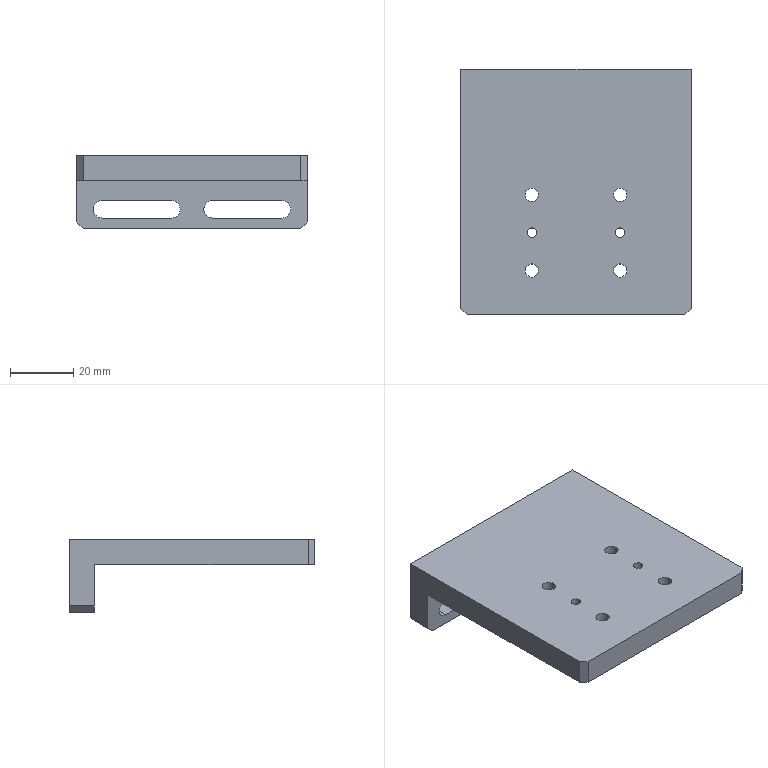Part | STEP file | 11-FG-SZ02611 | 1 solid | 34 faces | box 73 x 77.8 x 23 mm | volume 51259 mm3 | cylinder 18 | plane 16 | commonest cylinder face diameters 4.2 x8 5.5 x6 3 x4
STEP:
#1=CARTESIAN_POINT('',(-3.75,38.9,-9.));
#2=VERTEX_POINT('',#1);
#3=CARTESIAN_POINT('',(-6.5,38.9,-6.25));
#4=VERTEX_POINT('',#3);
#5=CARTESIAN_POINT('',(-6.5,38.9,-9.));
#6=DIRECTION('',(0.,-1.,0.));
#7=DIRECTION('',(0.,0.,-1.));
#8=AXIS2_PLACEMENT_3D('',#5,#6,#7);
#9=CIRCLE('',#8,2.75);
#10=EDGE_CURVE('',#2,#4,#9,.T.);
#11=ORIENTED_EDGE('',*,*,#10,.F.);
#12=CARTESIAN_POINT('',(-3.75,30.9,-9.));
#13=VERTEX_POINT('',#12);
#14=CARTESIAN_POINT('',(-3.75,53.9,-9.));
#15=DIRECTION('',(0.,-1.,0.));
#16=VECTOR('',#15,1000.);
#17=LINE('',#14,#16);
#18=EDGE_CURVE('',#2,#13,#17,.T.);
#19=ORIENTED_EDGE('',*,*,#18,.T.);
#20=CARTESIAN_POINT('',(-6.5,30.9,-6.25));
#21=VERTEX_POINT('',#20);
#22=CARTESIAN_POINT('',(-6.5,30.9,-9.));
#23=DIRECTION('',(0.,-1.,0.));
#24=DIRECTION('',(1.,0.,0.));
#25=AXIS2_PLACEMENT_3D('',#22,#23,#24);
#26=CIRCLE('',#25,2.75);
#27=EDGE_CURVE('',#13,#21,#26,.T.);
#28=ORIENTED_EDGE('',*,*,#27,.T.);
#29=CARTESIAN_POINT('',(-6.5,53.9,-6.25));
#30=DIRECTION('',(0.,-1.,0.));
#31=VECTOR('',#30,1000.);
#32=LINE('',#29,#31);
#33=EDGE_CURVE('',#4,#21,#32,.T.);
#34=ORIENTED_EDGE('',*,*,#33,.F.);
#35=EDGE_LOOP('',(#11,#19,#28,#34));
#36=FACE_OUTER_BOUND('',#35,.T.);
#37=CARTESIAN_POINT('',(-6.5,53.9,-9.));
#38=DIRECTION('',(0.,-1.,0.));
#39=DIRECTION('',(1.,0.,0.));
#40=AXIS2_PLACEMENT_3D('',#37,#38,#39);
#41=CYLINDRICAL_SURFACE('',#40,2.75);
#42=ADVANCED_FACE('',(#36),#41,.F.);
#43=CARTESIAN_POINT('',(-15.5,-12.9,8.));
#44=VERTEX_POINT('',#43);
#45=CARTESIAN_POINT('',(-12.5,-12.9,8.));
#46=VERTEX_POINT('',#45);
#47=CARTESIAN_POINT('',(-14.,-12.9,8.));
#48=DIRECTION('',(0.,0.,1.));
#49=DIRECTION('',(1.,0.,0.));
#50=AXIS2_PLACEMENT_3D('',#47,#48,#49);
#51=CIRCLE('',#50,1.5);
#52=EDGE_CURVE('',#44,#46,#51,.T.);
#53=ORIENTED_EDGE('',*,*,#52,.T.);
#54=CARTESIAN_POINT('',(-12.5,-12.9,0.));
#55=VERTEX_POINT('',#54);
#56=CARTESIAN_POINT('',(-12.5,-12.9,0.));
#57=DIRECTION('',(0.,0.,-1.));
#58=VECTOR('',#57,1000.);
#59=LINE('',#56,#58);
#60=EDGE_CURVE('',#46,#55,#59,.T.);
#61=ORIENTED_EDGE('',*,*,#60,.T.);
#62=CARTESIAN_POINT('',(-15.5,-12.9,0.));
#63=VERTEX_POINT('',#62);
#64=CARTESIAN_POINT('',(-14.,-12.9,0.));
#65=DIRECTION('',(0.,0.,-1.));
#66=DIRECTION('',(-1.,0.,0.));
#67=AXIS2_PLACEMENT_3D('',#64,#65,#66);
#68=CIRCLE('',#67,1.5);
#69=EDGE_CURVE('',#55,#63,#68,.T.);
#70=ORIENTED_EDGE('',*,*,#69,.T.);
#71=CARTESIAN_POINT('',(-15.5,-12.9,0.));
#72=DIRECTION('',(0.,0.,-1.));
#73=VECTOR('',#72,1000.);
#74=LINE('',#71,#73);
#75=EDGE_CURVE('',#44,#63,#74,.T.);
#76=ORIENTED_EDGE('',*,*,#75,.F.);
#77=EDGE_LOOP('',(#53,#61,#70,#76));
#78=FACE_OUTER_BOUND('',#77,.T.);
#79=CARTESIAN_POINT('',(-14.,-12.9,0.));
#80=DIRECTION('',(0.,0.,-1.));
#81=DIRECTION('',(-1.,0.,0.));
#82=AXIS2_PLACEMENT_3D('',#79,#80,#81);
#83=CYLINDRICAL_SURFACE('',#82,1.5);
#84=ADVANCED_FACE('',(#78),#83,.F.);
#85=CARTESIAN_POINT('',(12.5,-12.9,8.));
#86=VERTEX_POINT('',#85);
#87=CARTESIAN_POINT('',(15.5,-12.9,8.));
#88=VERTEX_POINT('',#87);
#89=CARTESIAN_POINT('',(14.,-12.9,8.));
#90=DIRECTION('',(0.,0.,1.));
#91=DIRECTION('',(1.,0.,0.));
#92=AXIS2_PLACEMENT_3D('',#89,#90,#91);
#93=CIRCLE('',#92,1.5);
#94=EDGE_CURVE('',#86,#88,#93,.T.);
#95=ORIENTED_EDGE('',*,*,#94,.T.);
#96=CARTESIAN_POINT('',(15.5,-12.9,0.));
#97=VERTEX_POINT('',#96);
#98=CARTESIAN_POINT('',(15.5,-12.9,0.));
#99=DIRECTION('',(0.,0.,-1.));
#100=VECTOR('',#99,1000.);
#101=LINE('',#98,#100);
#102=EDGE_CURVE('',#88,#97,#101,.T.);
#103=ORIENTED_EDGE('',*,*,#102,.T.);
#104=CARTESIAN_POINT('',(12.5,-12.9,0.));
#105=VERTEX_POINT('',#104);
#106=CARTESIAN_POINT('',(14.,-12.9,0.));
#107=DIRECTION('',(0.,0.,-1.));
#108=DIRECTION('',(-1.,0.,0.));
#109=AXIS2_PLACEMENT_3D('',#106,#107,#108);
#110=CIRCLE('',#109,1.5);
#111=EDGE_CURVE('',#97,#105,#110,.T.);
#112=ORIENTED_EDGE('',*,*,#111,.T.);
#113=CARTESIAN_POINT('',(12.5,-12.9,0.));
#114=DIRECTION('',(0.,0.,-1.));
#115=VECTOR('',#114,1000.);
#116=LINE('',#113,#115);
#117=EDGE_CURVE('',#86,#105,#116,.T.);
#118=ORIENTED_EDGE('',*,*,#117,.F.);
#119=EDGE_LOOP('',(#95,#103,#112,#118));
#120=FACE_OUTER_BOUND('',#119,.T.);
#121=CARTESIAN_POINT('',(14.,-12.9,0.));
#122=DIRECTION('',(0.,0.,-1.));
#123=DIRECTION('',(-1.,0.,0.));
#124=AXIS2_PLACEMENT_3D('',#121,#122,#123);
#125=CYLINDRICAL_SURFACE('',#124,1.5);
#126=ADVANCED_FACE('',(#120),#125,.F.);
#127=CARTESIAN_POINT('',(11.9,-24.9,0.));
#128=VERTEX_POINT('',#127);
#129=CARTESIAN_POINT('',(16.1,-24.9,0.));
#130=VERTEX_POINT('',#129);
#131=CARTESIAN_POINT('',(14.,-24.9,0.));
#132=DIRECTION('',(0.,0.,1.));
#133=DIRECTION('',(1.,0.,0.));
#134=AXIS2_PLACEMENT_3D('',#131,#132,#133);
#135=CIRCLE('',#134,2.1);
#136=EDGE_CURVE('',#128,#130,#135,.T.);
#137=ORIENTED_EDGE('',*,*,#136,.F.);
#138=CARTESIAN_POINT('',(11.9,-24.9,8.));
#139=VERTEX_POINT('',#138);
#140=CARTESIAN_POINT('',(11.9,-24.9,8.));
#141=DIRECTION('',(0.,0.,1.));
#142=VECTOR('',#141,1000.);
#143=LINE('',#140,#142);
#144=EDGE_CURVE('',#128,#139,#143,.T.);
#145=ORIENTED_EDGE('',*,*,#144,.T.);
#146=CARTESIAN_POINT('',(16.1,-24.9,8.));
#147=VERTEX_POINT('',#146);
#148=CARTESIAN_POINT('',(14.,-24.9,8.));
#149=DIRECTION('',(0.,0.,1.));
#150=DIRECTION('',(1.,0.,0.));
#151=AXIS2_PLACEMENT_3D('',#148,#149,#150);
#152=CIRCLE('',#151,2.1);
#153=EDGE_CURVE('',#139,#147,#152,.T.);
#154=ORIENTED_EDGE('',*,*,#153,.T.);
#155=CARTESIAN_POINT('',(16.1,-24.9,8.));
#156=DIRECTION('',(0.,0.,1.));
#157=VECTOR('',#156,1000.);
#158=LINE('',#155,#157);
#159=EDGE_CURVE('',#130,#147,#158,.T.);
#160=ORIENTED_EDGE('',*,*,#159,.F.);
#161=EDGE_LOOP('',(#137,#145,#154,#160));
#162=FACE_OUTER_BOUND('',#161,.T.);
#163=CARTESIAN_POINT('',(14.,-24.9,8.));
#164=DIRECTION('',(0.,0.,1.));
#165=DIRECTION('',(1.,0.,0.));
#166=AXIS2_PLACEMENT_3D('',#163,#164,#165);
#167=CYLINDRICAL_SURFACE('',#166,2.1);
#168=ADVANCED_FACE('',(#162),#167,.F.);
#169=CARTESIAN_POINT('',(11.9,-0.9,0.));
#170=VERTEX_POINT('',#169);
#171=CARTESIAN_POINT('',(16.1,-0.9,0.));
#172=VERTEX_POINT('',#171);
#173=CARTESIAN_POINT('',(14.,-0.9,0.));
#174=DIRECTION('',(0.,0.,1.));
#175=DIRECTION('',(1.,0.,0.));
#176=AXIS2_PLACEMENT_3D('',#173,#174,#175);
#177=CIRCLE('',#176,2.1);
#178=EDGE_CURVE('',#170,#172,#177,.T.);
#179=ORIENTED_EDGE('',*,*,#178,.F.);
#180=CARTESIAN_POINT('',(11.9,-0.9,8.));
#181=VERTEX_POINT('',#180);
#182=CARTESIAN_POINT('',(11.9,-0.9,8.));
#183=DIRECTION('',(0.,0.,1.));
#184=VECTOR('',#183,1000.);
#185=LINE('',#182,#184);
#186=EDGE_CURVE('',#170,#181,#185,.T.);
#187=ORIENTED_EDGE('',*,*,#186,.T.);
#188=CARTESIAN_POINT('',(16.1,-0.9,8.));
#189=VERTEX_POINT('',#188);
#190=CARTESIAN_POINT('',(14.,-0.9,8.));
#191=DIRECTION('',(0.,0.,1.));
#192=DIRECTION('',(1.,0.,0.));
#193=AXIS2_PLACEMENT_3D('',#190,#191,#192);
#194=CIRCLE('',#193,2.1);
#195=EDGE_CURVE('',#181,#189,#194,.T.);
#196=ORIENTED_EDGE('',*,*,#195,.T.);
#197=CARTESIAN_POINT('',(16.1,-0.9,8.));
#198=DIRECTION('',(0.,0.,1.));
#199=VECTOR('',#198,1000.);
#200=LINE('',#197,#199);
#201=EDGE_CURVE('',#172,#189,#200,.T.);
#202=ORIENTED_EDGE('',*,*,#201,.F.);
#203=EDGE_LOOP('',(#179,#187,#196,#202));
#204=FACE_OUTER_BOUND('',#203,.T.);
#205=CARTESIAN_POINT('',(14.,-0.9,8.));
#206=DIRECTION('',(0.,0.,1.));
#207=DIRECTION('',(1.,0.,0.));
#208=AXIS2_PLACEMENT_3D('',#205,#206,#207);
#209=CYLINDRICAL_SURFACE('',#208,2.1);
#210=ADVANCED_FACE('',(#204),#209,.F.);
#211=CARTESIAN_POINT('',(-16.1,-0.9,0.));
#212=VERTEX_POINT('',#211);
#213=CARTESIAN_POINT('',(-11.9,-0.9,0.));
#214=VERTEX_POINT('',#213);
#215=CARTESIAN_POINT('',(-14.,-0.9,0.));
#216=DIRECTION('',(0.,0.,1.));
#217=DIRECTION('',(1.,0.,0.));
#218=AXIS2_PLACEMENT_3D('',#215,#216,#217);
#219=CIRCLE('',#218,2.1);
#220=EDGE_CURVE('',#212,#214,#219,.T.);
#221=ORIENTED_EDGE('',*,*,#220,.F.);
#222=CARTESIAN_POINT('',(-16.1,-0.9,8.));
#223=VERTEX_POINT('',#222);
#224=CARTESIAN_POINT('',(-16.1,-0.9,8.));
#225=DIRECTION('',(0.,0.,1.));
#226=VECTOR('',#225,1000.);
#227=LINE('',#224,#226);
#228=EDGE_CURVE('',#212,#223,#227,.T.);
#229=ORIENTED_EDGE('',*,*,#228,.T.);
#230=CARTESIAN_POINT('',(-11.9,-0.9,8.));
#231=VERTEX_POINT('',#230);
#232=CARTESIAN_POINT('',(-14.,-0.9,8.));
#233=DIRECTION('',(0.,0.,1.));
#234=DIRECTION('',(1.,0.,0.));
#235=AXIS2_PLACEMENT_3D('',#232,#233,#234);
#236=CIRCLE('',#235,2.1);
#237=EDGE_CURVE('',#223,#231,#236,.T.);
#238=ORIENTED_EDGE('',*,*,#237,.T.);
#239=CARTESIAN_POINT('',(-11.9,-0.9,8.));
#240=DIRECTION('',(0.,0.,1.));
#241=VECTOR('',#240,1000.);
#242=LINE('',#239,#241);
#243=EDGE_CURVE('',#214,#231,#242,.T.);
#244=ORIENTED_EDGE('',*,*,#243,.F.);
#245=EDGE_LOOP('',(#221,#229,#238,#244));
#246=FACE_OUTER_BOUND('',#245,.T.);
#247=CARTESIAN_POINT('',(-14.,-0.9,8.));
#248=DIRECTION('',(0.,0.,1.));
#249=DIRECTION('',(1.,0.,0.));
#250=AXIS2_PLACEMENT_3D('',#247,#248,#249);
#251=CYLINDRICAL_SURFACE('',#250,2.1);
#252=ADVANCED_FACE('',(#246),#251,.F.);
#253=CARTESIAN_POINT('',(-16.1,-24.9,0.));
#254=VERTEX_POINT('',#253);
#255=CARTESIAN_POINT('',(-11.9,-24.9,0.));
#256=VERTEX_POINT('',#255);
#257=CARTESIAN_POINT('',(-14.,-24.9,0.));
#258=DIRECTION('',(0.,0.,1.));
#259=DIRECTION('',(1.,0.,0.));
#260=AXIS2_PLACEMENT_3D('',#257,#258,#259);
#261=CIRCLE('',#260,2.1);
#262=EDGE_CURVE('',#254,#256,#261,.T.);
#263=ORIENTED_EDGE('',*,*,#262,.F.);
#264=CARTESIAN_POINT('',(-16.1,-24.9,8.));
#265=VERTEX_POINT('',#264);
#266=CARTESIAN_POINT('',(-16.1,-24.9,8.));
#267=DIRECTION('',(0.,0.,1.));
#268=VECTOR('',#267,1000.);
#269=LINE('',#266,#268);
#270=EDGE_CURVE('',#254,#265,#269,.T.);
#271=ORIENTED_EDGE('',*,*,#270,.T.);
#272=CARTESIAN_POINT('',(-11.9,-24.9,8.));
#273=VERTEX_POINT('',#272);
#274=CARTESIAN_POINT('',(-14.,-24.9,8.));
#275=DIRECTION('',(0.,0.,1.));
#276=DIRECTION('',(1.,0.,0.));
#277=AXIS2_PLACEMENT_3D('',#274,#275,#276);
#278=CIRCLE('',#277,2.1);
#279=EDGE_CURVE('',#265,#273,#278,.T.);
#280=ORIENTED_EDGE('',*,*,#279,.T.);
#281=CARTESIAN_POINT('',(-11.9,-24.9,8.));
#282=DIRECTION('',(0.,0.,1.));
#283=VECTOR('',#282,1000.);
#284=LINE('',#281,#283);
#285=EDGE_CURVE('',#256,#273,#284,.T.);
#286=ORIENTED_EDGE('',*,*,#285,.F.);
#287=EDGE_LOOP('',(#263,#271,#280,#286));
#288=FACE_OUTER_BOUND('',#287,.T.);
#289=CARTESIAN_POINT('',(-14.,-24.9,8.));
#290=DIRECTION('',(0.,0.,1.));
#291=DIRECTION('',(1.,0.,0.));
#292=AXIS2_PLACEMENT_3D('',#289,#290,#291);
#293=CYLINDRICAL_SURFACE('',#292,2.1);
#294=ADVANCED_FACE('',(#288),#293,.F.);
#295=CARTESIAN_POINT('',(31.25,38.9,-9.));
#296=VERTEX_POINT('',#295);
#297=CARTESIAN_POINT('',(28.5,38.9,-6.25));
#298=VERTEX_POINT('',#297);
#299=CARTESIAN_POINT('',(28.5,38.9,-9.));
#300=DIRECTION('',(0.,-1.,0.));
#301=DIRECTION('',(0.,0.,-1.));
#302=AXIS2_PLACEMENT_3D('',#299,#300,#301);
#303=CIRCLE('',#302,2.75);
#304=EDGE_CURVE('',#296,#298,#303,.T.);
#305=ORIENTED_EDGE('',*,*,#304,.F.);
#306=CARTESIAN_POINT('',(31.25,30.9,-9.));
#307=VERTEX_POINT('',#306);
#308=CARTESIAN_POINT('',(31.25,47.9,-9.));
#309=DIRECTION('',(0.,-1.,0.));
#310=VECTOR('',#309,1000.);
#311=LINE('',#308,#310);
#312=EDGE_CURVE('',#296,#307,#311,.T.);
#313=ORIENTED_EDGE('',*,*,#312,.T.);
#314=CARTESIAN_POINT('',(28.5,30.9,-6.25));
#315=VERTEX_POINT('',#314);
#316=CARTESIAN_POINT('',(28.5,30.9,-9.));
#317=DIRECTION('',(0.,-1.,0.));
#318=DIRECTION('',(1.,0.,0.));
#319=AXIS2_PLACEMENT_3D('',#316,#317,#318);
#320=CIRCLE('',#319,2.75);
#321=EDGE_CURVE('',#307,#315,#320,.T.);
#322=ORIENTED_EDGE('',*,*,#321,.T.);
#323=CARTESIAN_POINT('',(28.5,47.9,-6.25));
#324=DIRECTION('',(0.,1.,0.));
#325=VECTOR('',#324,1000.);
#326=LINE('',#323,#325);
#327=EDGE_CURVE('',#315,#298,#326,.T.);
#328=ORIENTED_EDGE('',*,*,#327,.T.);
#329=EDGE_LOOP('',(#305,#313,#322,#328));
#330=FACE_OUTER_BOUND('',#329,.T.);
#331=CARTESIAN_POINT('',(28.5,47.9,-9.));
#332=DIRECTION('',(0.,-1.,0.));
#333=DIRECTION('',(1.,0.,0.));
#334=AXIS2_PLACEMENT_3D('',#331,#332,#333);
#335=CYLINDRICAL_SURFACE('',#334,2.75);
#336=ADVANCED_FACE('',(#330),#335,.F.);
#337=ORIENTED_EDGE('',*,*,#312,.F.);
#338=CARTESIAN_POINT('',(28.5,38.9,-11.75));
#339=VERTEX_POINT('',#338);
#340=CARTESIAN_POINT('',(28.5,38.9,-9.));
#341=DIRECTION('',(0.,-1.,0.));
#342=DIRECTION('',(0.,0.,-1.));
#343=AXIS2_PLACEMENT_3D('',#340,#341,#342);
#344=CIRCLE('',#343,2.75);
#345=EDGE_CURVE('',#339,#296,#344,.T.);
#346=ORIENTED_EDGE('',*,*,#345,.F.);
#347=CARTESIAN_POINT('',(28.5,30.9,-11.75));
#348=VERTEX_POINT('',#347);
#349=CARTESIAN_POINT('',(28.5,47.9,-11.75));
#350=DIRECTION('',(0.,1.,0.));
#351=VECTOR('',#350,1000.);
#352=LINE('',#349,#351);
#353=EDGE_CURVE('',#348,#339,#352,.T.);
#354=ORIENTED_EDGE('',*,*,#353,.F.);
#355=CARTESIAN_POINT('',(28.5,30.9,-9.));
#356=DIRECTION('',(0.,-1.,0.));
#357=DIRECTION('',(1.,0.,0.));
#358=AXIS2_PLACEMENT_3D('',#355,#356,#357);
#359=CIRCLE('',#358,2.75);
#360=EDGE_CURVE('',#348,#307,#359,.T.);
#361=ORIENTED_EDGE('',*,*,#360,.T.);
#362=EDGE_LOOP('',(#337,#346,#354,#361));
#363=FACE_OUTER_BOUND('',#362,.T.);
#364=CARTESIAN_POINT('',(28.5,47.9,-9.));
#365=DIRECTION('',(0.,-1.,0.));
#366=DIRECTION('',(1.,0.,0.));
#367=AXIS2_PLACEMENT_3D('',#364,#365,#366);
#368=CYLINDRICAL_SURFACE('',#367,2.75);
#369=ADVANCED_FACE('',(#363),#368,.F.);
#370=CARTESIAN_POINT('',(-28.5,30.9,-6.25));
#371=VERTEX_POINT('',#370);
#372=CARTESIAN_POINT('',(-28.5,38.9,-6.25));
#373=VERTEX_POINT('',#372);
#374=CARTESIAN_POINT('',(-28.5,47.9,-6.25));
#375=DIRECTION('',(0.,1.,0.));
#376=VECTOR('',#375,1000.);
#377=LINE('',#374,#376);
#378=EDGE_CURVE('',#371,#373,#377,.T.);
#379=ORIENTED_EDGE('',*,*,#378,.F.);
#380=CARTESIAN_POINT('',(-28.5,30.9,-11.75));
#381=VERTEX_POINT('',#380);
#382=CARTESIAN_POINT('',(-28.5,30.9,-9.));
#383=DIRECTION('',(0.,-1.,0.));
#384=DIRECTION('',(1.,0.,0.));
#385=AXIS2_PLACEMENT_3D('',#382,#383,#384);
#386=CIRCLE('',#385,2.75);
#387=EDGE_CURVE('',#371,#381,#386,.T.);
#388=ORIENTED_EDGE('',*,*,#387,.T.);
#389=CARTESIAN_POINT('',(-28.5,38.9,-11.75));
#390=VERTEX_POINT('',#389);
#391=CARTESIAN_POINT('',(-28.5,47.9,-11.75));
#392=DIRECTION('',(0.,1.,0.));
#393=VECTOR('',#392,1000.);
#394=LINE('',#391,#393);
#395=EDGE_CURVE('',#381,#390,#394,.T.);
#396=ORIENTED_EDGE('',*,*,#395,.T.);
#397=CARTESIAN_POINT('',(-28.5,38.9,-9.));
#398=DIRECTION('',(0.,-1.,0.));
#399=DIRECTION('',(0.,0.,-1.));
#400=AXIS2_PLACEMENT_3D('',#397,#398,#399);
#401=CIRCLE('',#400,2.75);
#402=EDGE_CURVE('',#373,#390,#401,.T.);
#403=ORIENTED_EDGE('',*,*,#402,.F.);
#404=EDGE_LOOP('',(#379,#388,#396,#403));
#405=FACE_OUTER_BOUND('',#404,.T.);
#406=CARTESIAN_POINT('',(-28.5,47.9,-9.));
#407=DIRECTION('',(0.,-1.,0.));
#408=DIRECTION('',(1.,0.,0.));
#409=AXIS2_PLACEMENT_3D('',#406,#407,#408);
#410=CYLINDRICAL_SURFACE('',#409,2.75);
#411=ADVANCED_FACE('',(#405),#410,.F.);
#412=CARTESIAN_POINT('',(-14.,-12.9,0.));
#413=DIRECTION('',(0.,0.,-1.));
#414=DIRECTION('',(-1.,0.,0.));
#415=AXIS2_PLACEMENT_3D('',#412,#413,#414);
#416=CIRCLE('',#415,1.5);
#417=EDGE_CURVE('',#63,#55,#416,.T.);
#418=ORIENTED_EDGE('',*,*,#417,.F.);
#419=ORIENTED_EDGE('',*,*,#69,.F.);
#420=EDGE_LOOP('',(#418,#419));
#421=FACE_BOUND('',#420,.T.);
#422=CARTESIAN_POINT('',(14.,-12.9,0.));
#423=DIRECTION('',(0.,0.,-1.));
#424=DIRECTION('',(-1.,0.,0.));
#425=AXIS2_PLACEMENT_3D('',#422,#423,#424);
#426=CIRCLE('',#425,1.5);
#427=EDGE_CURVE('',#105,#97,#426,.T.);
#428=ORIENTED_EDGE('',*,*,#427,.F.);
#429=ORIENTED_EDGE('',*,*,#111,.F.);
#430=EDGE_LOOP('',(#428,#429));
#431=FACE_BOUND('',#430,.T.);
#432=CARTESIAN_POINT('',(14.,-24.9,0.));
#433=DIRECTION('',(0.,0.,1.));
#434=DIRECTION('',(1.,0.,0.));
#435=AXIS2_PLACEMENT_3D('',#432,#433,#434);
#436=CIRCLE('',#435,2.1);
#437=EDGE_CURVE('',#130,#128,#436,.T.);
#438=ORIENTED_EDGE('',*,*,#437,.T.);
#439=ORIENTED_EDGE('',*,*,#136,.T.);
#440=EDGE_LOOP('',(#438,#439));
#441=FACE_BOUND('',#440,.T.);
#442=CARTESIAN_POINT('',(14.,-0.9,0.));
#443=DIRECTION('',(0.,0.,1.));
#444=DIRECTION('',(1.,0.,0.));
#445=AXIS2_PLACEMENT_3D('',#442,#443,#444);
#446=CIRCLE('',#445,2.1);
#447=EDGE_CURVE('',#172,#170,#446,.T.);
#448=ORIENTED_EDGE('',*,*,#447,.T.);
#449=ORIENTED_EDGE('',*,*,#178,.T.);
#450=EDGE_LOOP('',(#448,#449));
#451=FACE_BOUND('',#450,.T.);
#452=CARTESIAN_POINT('',(-14.,-0.9,0.));
#453=DIRECTION('',(0.,0.,1.));
#454=DIRECTION('',(1.,0.,0.));
#455=AXIS2_PLACEMENT_3D('',#452,#453,#454);
#456=CIRCLE('',#455,2.1);
#457=EDGE_CURVE('',#214,#212,#456,.T.);
#458=ORIENTED_EDGE('',*,*,#457,.T.);
#459=ORIENTED_EDGE('',*,*,#220,.T.);
#460=EDGE_LOOP('',(#458,#459));
#461=FACE_BOUND('',#460,.T.);
#462=CARTESIAN_POINT('',(-14.,-24.9,0.));
#463=DIRECTION('',(0.,0.,1.));
#464=DIRECTION('',(1.,0.,0.));
#465=AXIS2_PLACEMENT_3D('',#462,#463,#464);
#466=CIRCLE('',#465,2.1);
#467=EDGE_CURVE('',#256,#254,#466,.T.);
#468=ORIENTED_EDGE('',*,*,#467,.T.);
#469=ORIENTED_EDGE('',*,*,#262,.T.);
#470=EDGE_LOOP('',(#468,#469));
#471=FACE_BOUND('',#470,.T.);
#472=CARTESIAN_POINT('',(36.5,-36.9,0.));
#473=VERTEX_POINT('',#472);
#474=CARTESIAN_POINT('',(36.5,30.9,0.));
#475=VERTEX_POINT('',#474);
#476=CARTESIAN_POINT('',(36.5,38.9,0.));
#477=DIRECTION('',(0.,1.,0.));
#478=VECTOR('',#477,1000.);
#479=LINE('',#476,#478);
#480=EDGE_CURVE('',#473,#475,#479,.T.);
#481=ORIENTED_EDGE('',*,*,#480,.F.);
#482=CARTESIAN_POINT('',(34.5,-38.9,0.));
#483=VERTEX_POINT('',#482);
#484=CARTESIAN_POINT('',(36.5,-36.9,0.));
#485=DIRECTION('',(-0.7071,-0.7071,0.));
#486=VECTOR('',#485,1000.);
#487=LINE('',#484,#486);
#488=EDGE_CURVE('',#473,#483,#487,.T.);
#489=ORIENTED_EDGE('',*,*,#488,.T.);
#490=CARTESIAN_POINT('',(-34.5,-38.9,0.));
#491=VERTEX_POINT('',#490);
#492=CARTESIAN_POINT('',(-36.5,-38.9,0.));
#493=DIRECTION('',(1.,0.,0.));
#494=VECTOR('',#493,1000.);
#495=LINE('',#492,#494);
#496=EDGE_CURVE('',#491,#483,#495,.T.);
#497=ORIENTED_EDGE('',*,*,#496,.F.);
#498=CARTESIAN_POINT('',(-36.5,-36.9,0.));
#499=VERTEX_POINT('',#498);
#500=CARTESIAN_POINT('',(-34.5,-38.9,0.));
#501=DIRECTION('',(-0.7071,0.7071,0.));
#502=VECTOR('',#501,1000.);
#503=LINE('',#500,#502);
#504=EDGE_CURVE('',#491,#499,#503,.T.);
#505=ORIENTED_EDGE('',*,*,#504,.T.);
#506=CARTESIAN_POINT('',(-36.5,30.9,0.));
#507=VERTEX_POINT('',#506);
#508=CARTESIAN_POINT('',(-36.5,38.9,0.));
#509=DIRECTION('',(0.,-1.,0.));
#510=VECTOR('',#509,1000.);
#511=LINE('',#508,#510);
#512=EDGE_CURVE('',#507,#499,#511,.T.);
#513=ORIENTED_EDGE('',*,*,#512,.F.);
#514=CARTESIAN_POINT('',(-36.5,30.9,0.));
#515=DIRECTION('',(-1.,0.,0.));
#516=VECTOR('',#515,1000.);
#517=LINE('',#514,#516);
#518=EDGE_CURVE('',#475,#507,#517,.T.);
#519=ORIENTED_EDGE('',*,*,#518,.F.);
#520=EDGE_LOOP('',(#481,#489,#497,#505,#513,#519));
#521=FACE_OUTER_BOUND('',#520,.T.);
#522=CARTESIAN_POINT('',(0.,0.,0.));
#523=DIRECTION('',(0.,0.,1.));
#524=DIRECTION('',(1.,0.,0.));
#525=AXIS2_PLACEMENT_3D('',#522,#523,#524);
#526=PLANE('',#525);
#527=ADVANCED_FACE('',(#421,#431,#441,#451,#461,#471,#521),#526,.F.);
#528=CARTESIAN_POINT('',(36.5,30.9,-13.));
#529=VERTEX_POINT('',#528);
#530=CARTESIAN_POINT('',(36.5,30.9,-15.));
#531=DIRECTION('',(0.,0.,1.));
#532=VECTOR('',#531,1000.);
#533=LINE('',#530,#532);
#534=EDGE_CURVE('',#529,#475,#533,.T.);
#535=ORIENTED_EDGE('',*,*,#534,.F.);
#536=CARTESIAN_POINT('',(36.5,38.9,-13.));
#537=VERTEX_POINT('',#536);
#538=CARTESIAN_POINT('',(36.5,38.9,-13.));
#539=DIRECTION('',(0.,1.,0.));
#540=VECTOR('',#539,1000.);
#541=LINE('',#538,#540);
#542=EDGE_CURVE('',#529,#537,#541,.T.);
#543=ORIENTED_EDGE('',*,*,#542,.T.);
#544=CARTESIAN_POINT('',(36.5,38.9,8.));
#545=VERTEX_POINT('',#544);
#546=CARTESIAN_POINT('',(36.5,38.9,8.));
#547=DIRECTION('',(0.,0.,-1.));
#548=VECTOR('',#547,1000.);
#549=LINE('',#546,#548);
#550=EDGE_CURVE('',#545,#537,#549,.T.);
#551=ORIENTED_EDGE('',*,*,#550,.F.);
#552=CARTESIAN_POINT('',(36.5,-36.9,8.));
#553=VERTEX_POINT('',#552);
#554=CARTESIAN_POINT('',(36.5,38.9,8.));
#555=DIRECTION('',(0.,1.,0.));
#556=VECTOR('',#555,1000.);
#557=LINE('',#554,#556);
#558=EDGE_CURVE('',#553,#545,#557,.T.);
#559=ORIENTED_EDGE('',*,*,#558,.F.);
#560=CARTESIAN_POINT('',(36.5,-36.9,8.));
#561=DIRECTION('',(0.,0.,-1.));
#562=VECTOR('',#561,1000.);
#563=LINE('',#560,#562);
#564=EDGE_CURVE('',#553,#473,#563,.T.);
#565=ORIENTED_EDGE('',*,*,#564,.T.);
#566=ORIENTED_EDGE('',*,*,#480,.T.);
#567=EDGE_LOOP('',(#535,#543,#551,#559,#565,#566));
#568=FACE_OUTER_BOUND('',#567,.T.);
#569=CARTESIAN_POINT('',(36.5,38.9,8.));
#570=DIRECTION('',(-1.,0.,0.));
#571=DIRECTION('',(0.,-1.,0.));
#572=AXIS2_PLACEMENT_3D('',#569,#570,#571);
#573=PLANE('',#572);
#574=ADVANCED_FACE('',(#568),#573,.F.);
#575=CARTESIAN_POINT('',(6.5,38.9,-6.25));
#576=VERTEX_POINT('',#575);
#577=CARTESIAN_POINT('',(6.5,38.9,-11.75));
#578=VERTEX_POINT('',#577);
#579=CARTESIAN_POINT('',(6.5,38.9,-9.));
#580=DIRECTION('',(0.,-1.,0.));
#581=DIRECTION('',(0.,0.,-1.));
#582=AXIS2_PLACEMENT_3D('',#579,#580,#581);
#583=CIRCLE('',#582,2.75);
#584=EDGE_CURVE('',#576,#578,#583,.T.);
#585=ORIENTED_EDGE('',*,*,#584,.T.);
#586=CARTESIAN_POINT('',(-36.5,38.9,-11.75));
#587=DIRECTION('',(1.,0.,0.));
#588=VECTOR('',#587,1000.);
#589=LINE('',#586,#588);
#590=EDGE_CURVE('',#578,#339,#589,.T.);
#591=ORIENTED_EDGE('',*,*,#590,.T.);
#592=ORIENTED_EDGE('',*,*,#345,.T.);
#593=ORIENTED_EDGE('',*,*,#304,.T.);
#594=CARTESIAN_POINT('',(-36.5,38.9,-6.25));
#595=DIRECTION('',(-1.,0.,0.));
#596=VECTOR('',#595,1000.);
#597=LINE('',#594,#596);
#598=EDGE_CURVE('',#298,#576,#597,.T.);
#599=ORIENTED_EDGE('',*,*,#598,.T.);
#600=EDGE_LOOP('',(#585,#591,#592,#593,#599));
#601=FACE_BOUND('',#600,.T.);
#602=CARTESIAN_POINT('',(-6.5,38.9,-11.75));
#603=VERTEX_POINT('',#602);
#604=CARTESIAN_POINT('',(-6.5,38.9,-9.));
#605=DIRECTION('',(0.,-1.,0.));
#606=DIRECTION('',(0.,0.,-1.));
#607=AXIS2_PLACEMENT_3D('',#604,#605,#606);
#608=CIRCLE('',#607,2.75);
#609=EDGE_CURVE('',#603,#2,#608,.T.);
#610=ORIENTED_EDGE('',*,*,#609,.T.);
#611=ORIENTED_EDGE('',*,*,#10,.T.);
#612=CARTESIAN_POINT('',(-36.5,38.9,-6.25));
#613=DIRECTION('',(-1.,0.,0.));
#614=VECTOR('',#613,1000.);
#615=LINE('',#612,#614);
#616=EDGE_CURVE('',#4,#373,#615,.T.);
#617=ORIENTED_EDGE('',*,*,#616,.T.);
#618=ORIENTED_EDGE('',*,*,#402,.T.);
#619=CARTESIAN_POINT('',(-36.5,38.9,-11.75));
#620=DIRECTION('',(1.,0.,0.));
#621=VECTOR('',#620,1000.);
#622=LINE('',#619,#621);
#623=EDGE_CURVE('',#390,#603,#622,.T.);
#624=ORIENTED_EDGE('',*,*,#623,.T.);
#625=EDGE_LOOP('',(#610,#611,#617,#618,#624));
#626=FACE_BOUND('',#625,.T.);
#627=CARTESIAN_POINT('',(-34.5,38.9,-15.));
#628=VERTEX_POINT('',#627);
#629=CARTESIAN_POINT('',(34.5,38.9,-15.));
#630=VERTEX_POINT('',#629);
#631=CARTESIAN_POINT('',(-36.5,38.9,-15.));
#632=DIRECTION('',(1.,0.,0.));
#633=VECTOR('',#632,1000.);
#634=LINE('',#631,#633);
#635=EDGE_CURVE('',#628,#630,#634,.T.);
#636=ORIENTED_EDGE('',*,*,#635,.F.);
#637=CARTESIAN_POINT('',(-36.5,38.9,-13.));
#638=VERTEX_POINT('',#637);
#639=CARTESIAN_POINT('',(-34.5,38.9,-15.));
#640=DIRECTION('',(-0.7071,0.,0.7071));
#641=VECTOR('',#640,1000.);
#642=LINE('',#639,#641);
#643=EDGE_CURVE('',#628,#638,#642,.T.);
#644=ORIENTED_EDGE('',*,*,#643,.T.);
#645=CARTESIAN_POINT('',(-36.5,38.9,8.));
#646=VERTEX_POINT('',#645);
#647=CARTESIAN_POINT('',(-36.5,38.9,8.));
#648=DIRECTION('',(0.,0.,-1.));
#649=VECTOR('',#648,1000.);
#650=LINE('',#647,#649);
#651=EDGE_CURVE('',#646,#638,#650,.T.);
#652=ORIENTED_EDGE('',*,*,#651,.F.);
#653=CARTESIAN_POINT('',(-36.5,38.9,8.));
#654=DIRECTION('',(-1.,0.,0.));
#655=VECTOR('',#654,1000.);
#656=LINE('',#653,#655);
#657=EDGE_CURVE('',#545,#646,#656,.T.);
#658=ORIENTED_EDGE('',*,*,#657,.F.);
#659=ORIENTED_EDGE('',*,*,#550,.T.);
#660=CARTESIAN_POINT('',(34.5,38.9,-15.));
#661=DIRECTION('',(-0.7071,0.,-0.7071));
#662=VECTOR('',#661,1000.);
#663=LINE('',#660,#662);
#664=EDGE_CURVE('',#537,#630,#663,.T.);
#665=ORIENTED_EDGE('',*,*,#664,.T.);
#666=EDGE_LOOP('',(#636,#644,#652,#658,#659,#665));
#667=FACE_OUTER_BOUND('',#666,.T.);
#668=CARTESIAN_POINT('',(-36.5,38.9,8.));
#669=DIRECTION('',(0.,-1.,0.));
#670=DIRECTION('',(0.,0.,-1.));
#671=AXIS2_PLACEMENT_3D('',#668,#669,#670);
#672=PLANE('',#671);
#673=ADVANCED_FACE('',(#601,#626,#667),#672,.F.);
#674=ORIENTED_EDGE('',*,*,#651,.T.);
#675=CARTESIAN_POINT('',(-36.5,30.9,-13.));
#676=VERTEX_POINT('',#675);
#677=CARTESIAN_POINT('',(-36.5,38.9,-13.));
#678=DIRECTION('',(0.,-1.,0.));
#679=VECTOR('',#678,1000.);
#680=LINE('',#677,#679);
#681=EDGE_CURVE('',#638,#676,#680,.T.);
#682=ORIENTED_EDGE('',*,*,#681,.T.);
#683=CARTESIAN_POINT('',(-36.5,30.9,-15.));
#684=DIRECTION('',(0.,0.,1.));
#685=VECTOR('',#684,1000.);
#686=LINE('',#683,#685);
#687=EDGE_CURVE('',#676,#507,#686,.T.);
#688=ORIENTED_EDGE('',*,*,#687,.T.);
#689=ORIENTED_EDGE('',*,*,#512,.T.);
#690=CARTESIAN_POINT('',(-36.5,-36.9,8.));
#691=VERTEX_POINT('',#690);
#692=CARTESIAN_POINT('',(-36.5,-36.9,8.));
#693=DIRECTION('',(0.,0.,1.));
#694=VECTOR('',#693,1000.);
#695=LINE('',#692,#694);
#696=EDGE_CURVE('',#499,#691,#695,.T.);
#697=ORIENTED_EDGE('',*,*,#696,.T.);
#698=CARTESIAN_POINT('',(-36.5,38.9,8.));
#699=DIRECTION('',(0.,-1.,0.));
#700=VECTOR('',#699,1000.);
#701=LINE('',#698,#700);
#702=EDGE_CURVE('',#646,#691,#701,.T.);
#703=ORIENTED_EDGE('',*,*,#702,.F.);
#704=EDGE_LOOP('',(#674,#682,#688,#689,#697,#703));
#705=FACE_OUTER_BOUND('',#704,.T.);
#706=CARTESIAN_POINT('',(-36.5,38.9,8.));
#707=DIRECTION('',(1.,0.,0.));
#708=DIRECTION('',(0.,1.,0.));
#709=AXIS2_PLACEMENT_3D('',#706,#707,#708);
#710=PLANE('',#709);
#711=ADVANCED_FACE('',(#705),#710,.F.);
#712=ORIENTED_EDGE('',*,*,#496,.T.);
#713=CARTESIAN_POINT('',(34.5,-38.9,8.));
#714=VERTEX_POINT('',#713);
#715=CARTESIAN_POINT('',(34.5,-38.9,8.));
#716=DIRECTION('',(0.,0.,1.));
#717=VECTOR('',#716,1000.);
#718=LINE('',#715,#717);
#719=EDGE_CURVE('',#483,#714,#718,.T.);
#720=ORIENTED_EDGE('',*,*,#719,.T.);
#721=CARTESIAN_POINT('',(-34.5,-38.9,8.));
#722=VERTEX_POINT('',#721);
#723=CARTESIAN_POINT('',(-36.5,-38.9,8.));
#724=DIRECTION('',(1.,0.,0.));
#725=VECTOR('',#724,1000.);
#726=LINE('',#723,#725);
#727=EDGE_CURVE('',#722,#714,#726,.T.);
#728=ORIENTED_EDGE('',*,*,#727,.F.);
#729=CARTESIAN_POINT('',(-34.5,-38.9,8.));
#730=DIRECTION('',(0.,0.,-1.));
#731=VECTOR('',#730,1000.);
#732=LINE('',#729,#731);
#733=EDGE_CURVE('',#722,#491,#732,.T.);
#734=ORIENTED_EDGE('',*,*,#733,.T.);
#735=EDGE_LOOP('',(#712,#720,#728,#734));
#736=FACE_OUTER_BOUND('',#735,.T.);
#737=CARTESIAN_POINT('',(-36.5,-38.9,8.));
#738=DIRECTION('',(0.,1.,0.));
#739=DIRECTION('',(0.,0.,1.));
#740=AXIS2_PLACEMENT_3D('',#737,#738,#739);
#741=PLANE('',#740);
#742=ADVANCED_FACE('',(#736),#741,.F.);
#743=ORIENTED_EDGE('',*,*,#52,.F.);
#744=CARTESIAN_POINT('',(-14.,-12.9,8.));
#745=DIRECTION('',(0.,0.,1.));
#746=DIRECTION('',(1.,0.,0.));
#747=AXIS2_PLACEMENT_3D('',#744,#745,#746);
#748=CIRCLE('',#747,1.5);
#749=EDGE_CURVE('',#46,#44,#748,.T.);
#750=ORIENTED_EDGE('',*,*,#749,.F.);
#751=EDGE_LOOP('',(#743,#750));
#752=FACE_BOUND('',#751,.T.);
#753=ORIENTED_EDGE('',*,*,#94,.F.);
#754=CARTESIAN_POINT('',(14.,-12.9,8.));
#755=DIRECTION('',(0.,0.,1.));
#756=DIRECTION('',(1.,0.,0.));
#757=AXIS2_PLACEMENT_3D('',#754,#755,#756);
#758=CIRCLE('',#757,1.5);
#759=EDGE_CURVE('',#88,#86,#758,.T.);
#760=ORIENTED_EDGE('',*,*,#759,.F.);
#761=EDGE_LOOP('',(#753,#760));
#762=FACE_BOUND('',#761,.T.);
#763=CARTESIAN_POINT('',(14.,-24.9,8.));
#764=DIRECTION('',(0.,0.,1.));
#765=DIRECTION('',(1.,0.,0.));
#766=AXIS2_PLACEMENT_3D('',#763,#764,#765);
#767=CIRCLE('',#766,2.1);
#768=EDGE_CURVE('',#147,#139,#767,.T.);
#769=ORIENTED_EDGE('',*,*,#768,.F.);
#770=ORIENTED_EDGE('',*,*,#153,.F.);
#771=EDGE_LOOP('',(#769,#770));
#772=FACE_BOUND('',#771,.T.);
#773=CARTESIAN_POINT('',(14.,-0.9,8.));
#774=DIRECTION('',(0.,0.,1.));
#775=DIRECTION('',(1.,0.,0.));
#776=AXIS2_PLACEMENT_3D('',#773,#774,#775);
#777=CIRCLE('',#776,2.1);
#778=EDGE_CURVE('',#189,#181,#777,.T.);
#779=ORIENTED_EDGE('',*,*,#778,.F.);
#780=ORIENTED_EDGE('',*,*,#195,.F.);
#781=EDGE_LOOP('',(#779,#780));
#782=FACE_BOUND('',#781,.T.);
#783=CARTESIAN_POINT('',(-14.,-0.9,8.));
#784=DIRECTION('',(0.,0.,1.));
#785=DIRECTION('',(1.,0.,0.));
#786=AXIS2_PLACEMENT_3D('',#783,#784,#785);
#787=CIRCLE('',#786,2.1);
#788=EDGE_CURVE('',#231,#223,#787,.T.);
#789=ORIENTED_EDGE('',*,*,#788,.F.);
#790=ORIENTED_EDGE('',*,*,#237,.F.);
#791=EDGE_LOOP('',(#789,#790));
#792=FACE_BOUND('',#791,.T.);
#793=CARTESIAN_POINT('',(-14.,-24.9,8.));
#794=DIRECTION('',(0.,0.,1.));
#795=DIRECTION('',(1.,0.,0.));
#796=AXIS2_PLACEMENT_3D('',#793,#794,#795);
#797=CIRCLE('',#796,2.1);
#798=EDGE_CURVE('',#273,#265,#797,.T.);
#799=ORIENTED_EDGE('',*,*,#798,.F.);
#800=ORIENTED_EDGE('',*,*,#279,.F.);
#801=EDGE_LOOP('',(#799,#800));
#802=FACE_BOUND('',#801,.T.);
#803=ORIENTED_EDGE('',*,*,#727,.T.);
#804=CARTESIAN_POINT('',(36.7,-36.7,8.));
#805=DIRECTION('',(0.7071,0.7071,0.));
#806=VECTOR('',#805,1000.);
#807=LINE('',#804,#806);
#808=EDGE_CURVE('',#714,#553,#807,.T.);
#809=ORIENTED_EDGE('',*,*,#808,.T.);
#810=ORIENTED_EDGE('',*,*,#558,.T.);
#811=ORIENTED_EDGE('',*,*,#657,.T.);
#812=ORIENTED_EDGE('',*,*,#702,.T.);
#813=CARTESIAN_POINT('',(-36.7,-36.7,8.));
#814=DIRECTION('',(0.7071,-0.7071,0.));
#815=VECTOR('',#814,1000.);
#816=LINE('',#813,#815);
#817=EDGE_CURVE('',#691,#722,#816,.T.);
#818=ORIENTED_EDGE('',*,*,#817,.T.);
#819=EDGE_LOOP('',(#803,#809,#810,#811,#812,#818));
#820=FACE_OUTER_BOUND('',#819,.T.);
#821=CARTESIAN_POINT('',(0.,0.,8.));
#822=DIRECTION('',(0.,0.,1.));
#823=DIRECTION('',(1.,0.,0.));
#824=AXIS2_PLACEMENT_3D('',#821,#822,#823);
#825=PLANE('',#824);
#826=ADVANCED_FACE('',(#752,#762,#772,#782,#792,#802,#820),#825,.T.);
#827=ORIENTED_EDGE('',*,*,#360,.F.);
#828=CARTESIAN_POINT('',(6.5,30.9,-11.75));
#829=VERTEX_POINT('',#828);
#830=CARTESIAN_POINT('',(28.5,30.9,-11.75));
#831=DIRECTION('',(1.,0.,0.));
#832=VECTOR('',#831,1000.);
#833=LINE('',#830,#832);
#834=EDGE_CURVE('',#829,#348,#833,.T.);
#835=ORIENTED_EDGE('',*,*,#834,.F.);
#836=CARTESIAN_POINT('',(6.5,30.9,-6.25));
#837=VERTEX_POINT('',#836);
#838=CARTESIAN_POINT('',(6.5,30.9,-9.));
#839=DIRECTION('',(0.,-1.,0.));
#840=DIRECTION('',(1.,0.,0.));
#841=AXIS2_PLACEMENT_3D('',#838,#839,#840);
#842=CIRCLE('',#841,2.75);
#843=EDGE_CURVE('',#837,#829,#842,.T.);
#844=ORIENTED_EDGE('',*,*,#843,.F.);
#845=CARTESIAN_POINT('',(28.5,30.9,-6.25));
#846=DIRECTION('',(-1.,0.,0.));
#847=VECTOR('',#846,1000.);
#848=LINE('',#845,#847);
#849=EDGE_CURVE('',#315,#837,#848,.T.);
#850=ORIENTED_EDGE('',*,*,#849,.F.);
#851=ORIENTED_EDGE('',*,*,#321,.F.);
#852=EDGE_LOOP('',(#827,#835,#844,#850,#851));
#853=FACE_BOUND('',#852,.T.);
#854=ORIENTED_EDGE('',*,*,#387,.F.);
#855=CARTESIAN_POINT('',(-28.5,30.9,-6.25));
#856=DIRECTION('',(-1.,0.,0.));
#857=VECTOR('',#856,1000.);
#858=LINE('',#855,#857);
#859=EDGE_CURVE('',#21,#371,#858,.T.);
#860=ORIENTED_EDGE('',*,*,#859,.F.);
#861=ORIENTED_EDGE('',*,*,#27,.F.);
#862=CARTESIAN_POINT('',(-6.5,30.9,-11.75));
#863=VERTEX_POINT('',#862);
#864=CARTESIAN_POINT('',(-6.5,30.9,-9.));
#865=DIRECTION('',(0.,-1.,0.));
#866=DIRECTION('',(1.,0.,0.));
#867=AXIS2_PLACEMENT_3D('',#864,#865,#866);
#868=CIRCLE('',#867,2.75);
#869=EDGE_CURVE('',#863,#13,#868,.T.);
#870=ORIENTED_EDGE('',*,*,#869,.F.);
#871=CARTESIAN_POINT('',(-28.5,30.9,-11.75));
#872=DIRECTION('',(1.,0.,0.));
#873=VECTOR('',#872,1000.);
#874=LINE('',#871,#873);
#875=EDGE_CURVE('',#381,#863,#874,.T.);
#876=ORIENTED_EDGE('',*,*,#875,.F.);
#877=EDGE_LOOP('',(#854,#860,#861,#870,#876));
#878=FACE_BOUND('',#877,.T.);
#879=ORIENTED_EDGE('',*,*,#687,.F.);
#880=CARTESIAN_POINT('',(-34.5,30.9,-15.));
#881=VERTEX_POINT('',#880);
#882=CARTESIAN_POINT('',(-34.5,30.9,-15.));
#883=DIRECTION('',(0.7071,0.,-0.7071));
#884=VECTOR('',#883,1000.);
#885=LINE('',#882,#884);
#886=EDGE_CURVE('',#676,#881,#885,.T.);
#887=ORIENTED_EDGE('',*,*,#886,.T.);
#888=CARTESIAN_POINT('',(34.5,30.9,-15.));
#889=VERTEX_POINT('',#888);
#890=CARTESIAN_POINT('',(-36.5,30.9,-15.));
#891=DIRECTION('',(-1.,0.,0.));
#892=VECTOR('',#891,1000.);
#893=LINE('',#890,#892);
#894=EDGE_CURVE('',#889,#881,#893,.T.);
#895=ORIENTED_EDGE('',*,*,#894,.F.);
#896=CARTESIAN_POINT('',(34.5,30.9,-15.));
#897=DIRECTION('',(0.7071,0.,0.7071));
#898=VECTOR('',#897,1000.);
#899=LINE('',#896,#898);
#900=EDGE_CURVE('',#889,#529,#899,.T.);
#901=ORIENTED_EDGE('',*,*,#900,.T.);
#902=ORIENTED_EDGE('',*,*,#534,.T.);
#903=ORIENTED_EDGE('',*,*,#518,.T.);
#904=EDGE_LOOP('',(#879,#887,#895,#901,#902,#903));
#905=FACE_OUTER_BOUND('',#904,.T.);
#906=CARTESIAN_POINT('',(-36.5,30.9,-15.));
#907=DIRECTION('',(0.,1.,0.));
#908=DIRECTION('',(-1.,0.,0.));
#909=AXIS2_PLACEMENT_3D('',#906,#907,#908);
#910=PLANE('',#909);
#911=ADVANCED_FACE('',(#853,#878,#905),#910,.F.);
#912=ORIENTED_EDGE('',*,*,#894,.T.);
#913=CARTESIAN_POINT('',(-34.5,0.,-15.));
#914=DIRECTION('',(0.,1.,0.));
#915=VECTOR('',#914,1000.);
#916=LINE('',#913,#915);
#917=EDGE_CURVE('',#881,#628,#916,.T.);
#918=ORIENTED_EDGE('',*,*,#917,.T.);
#919=ORIENTED_EDGE('',*,*,#635,.T.);
#920=CARTESIAN_POINT('',(34.5,0.,-15.));
#921=DIRECTION('',(0.,-1.,0.));
#922=VECTOR('',#921,1000.);
#923=LINE('',#920,#922);
#924=EDGE_CURVE('',#630,#889,#923,.T.);
#925=ORIENTED_EDGE('',*,*,#924,.T.);
#926=EDGE_LOOP('',(#912,#918,#919,#925));
#927=FACE_OUTER_BOUND('',#926,.T.);
#928=CARTESIAN_POINT('',(0.,0.,-15.));
#929=DIRECTION('',(0.,0.,1.));
#930=DIRECTION('',(1.,0.,0.));
#931=AXIS2_PLACEMENT_3D('',#928,#929,#930);
#932=PLANE('',#931);
#933=ADVANCED_FACE('',(#927),#932,.F.);
#934=ORIENTED_EDGE('',*,*,#270,.F.);
#935=ORIENTED_EDGE('',*,*,#467,.F.);
#936=ORIENTED_EDGE('',*,*,#285,.T.);
#937=ORIENTED_EDGE('',*,*,#798,.T.);
#938=EDGE_LOOP('',(#934,#935,#936,#937));
#939=FACE_OUTER_BOUND('',#938,.T.);
#940=CARTESIAN_POINT('',(-14.,-24.9,8.));
#941=DIRECTION('',(0.,0.,1.));
#942=DIRECTION('',(1.,0.,0.));
#943=AXIS2_PLACEMENT_3D('',#940,#941,#942);
#944=CYLINDRICAL_SURFACE('',#943,2.1);
#945=ADVANCED_FACE('',(#939),#944,.F.);
#946=ORIENTED_EDGE('',*,*,#228,.F.);
#947=ORIENTED_EDGE('',*,*,#457,.F.);
#948=ORIENTED_EDGE('',*,*,#243,.T.);
#949=ORIENTED_EDGE('',*,*,#788,.T.);
#950=EDGE_LOOP('',(#946,#947,#948,#949));
#951=FACE_OUTER_BOUND('',#950,.T.);
#952=CARTESIAN_POINT('',(-14.,-0.9,8.));
#953=DIRECTION('',(0.,0.,1.));
#954=DIRECTION('',(1.,0.,0.));
#955=AXIS2_PLACEMENT_3D('',#952,#953,#954);
#956=CYLINDRICAL_SURFACE('',#955,2.1);
#957=ADVANCED_FACE('',(#951),#956,.F.);
#958=ORIENTED_EDGE('',*,*,#186,.F.);
#959=ORIENTED_EDGE('',*,*,#447,.F.);
#960=ORIENTED_EDGE('',*,*,#201,.T.);
#961=ORIENTED_EDGE('',*,*,#778,.T.);
#962=EDGE_LOOP('',(#958,#959,#960,#961));
#963=FACE_OUTER_BOUND('',#962,.T.);
#964=CARTESIAN_POINT('',(14.,-0.9,8.));
#965=DIRECTION('',(0.,0.,1.));
#966=DIRECTION('',(1.,0.,0.));
#967=AXIS2_PLACEMENT_3D('',#964,#965,#966);
#968=CYLINDRICAL_SURFACE('',#967,2.1);
#969=ADVANCED_FACE('',(#963),#968,.F.);
#970=ORIENTED_EDGE('',*,*,#144,.F.);
#971=ORIENTED_EDGE('',*,*,#437,.F.);
#972=ORIENTED_EDGE('',*,*,#159,.T.);
#973=ORIENTED_EDGE('',*,*,#768,.T.);
#974=EDGE_LOOP('',(#970,#971,#972,#973));
#975=FACE_OUTER_BOUND('',#974,.T.);
#976=CARTESIAN_POINT('',(14.,-24.9,8.));
#977=DIRECTION('',(0.,0.,1.));
#978=DIRECTION('',(1.,0.,0.));
#979=AXIS2_PLACEMENT_3D('',#976,#977,#978);
#980=CYLINDRICAL_SURFACE('',#979,2.1);
#981=ADVANCED_FACE('',(#975),#980,.F.);
#982=ORIENTED_EDGE('',*,*,#102,.F.);
#983=ORIENTED_EDGE('',*,*,#759,.T.);
#984=ORIENTED_EDGE('',*,*,#117,.T.);
#985=ORIENTED_EDGE('',*,*,#427,.T.);
#986=EDGE_LOOP('',(#982,#983,#984,#985));
#987=FACE_OUTER_BOUND('',#986,.T.);
#988=CARTESIAN_POINT('',(14.,-12.9,0.));
#989=DIRECTION('',(0.,0.,-1.));
#990=DIRECTION('',(-1.,0.,0.));
#991=AXIS2_PLACEMENT_3D('',#988,#989,#990);
#992=CYLINDRICAL_SURFACE('',#991,1.5);
#993=ADVANCED_FACE('',(#987),#992,.F.);
#994=ORIENTED_EDGE('',*,*,#60,.F.);
#995=ORIENTED_EDGE('',*,*,#749,.T.);
#996=ORIENTED_EDGE('',*,*,#75,.T.);
#997=ORIENTED_EDGE('',*,*,#417,.T.);
#998=EDGE_LOOP('',(#994,#995,#996,#997));
#999=FACE_OUTER_BOUND('',#998,.T.);
#1000=CARTESIAN_POINT('',(-14.,-12.9,0.));
#1001=DIRECTION('',(0.,0.,-1.));
#1002=DIRECTION('',(-1.,0.,0.));
#1003=AXIS2_PLACEMENT_3D('',#1000,#1001,#1002);
#1004=CYLINDRICAL_SURFACE('',#1003,1.5);
#1005=ADVANCED_FACE('',(#999),#1004,.F.);
#1006=ORIENTED_EDGE('',*,*,#886,.F.);
#1007=ORIENTED_EDGE('',*,*,#681,.F.);
#1008=ORIENTED_EDGE('',*,*,#643,.F.);
#1009=ORIENTED_EDGE('',*,*,#917,.F.);
#1010=EDGE_LOOP('',(#1006,#1007,#1008,#1009));
#1011=FACE_OUTER_BOUND('',#1010,.T.);
#1012=CARTESIAN_POINT('',(-34.5,0.,-15.));
#1013=DIRECTION('',(0.7071,0.,0.7071));
#1014=DIRECTION('',(0.,1.,0.));
#1015=AXIS2_PLACEMENT_3D('',#1012,#1013,#1014);
#1016=PLANE('',#1015);
#1017=ADVANCED_FACE('',(#1011),#1016,.F.);
#1018=ORIENTED_EDGE('',*,*,#664,.F.);
#1019=ORIENTED_EDGE('',*,*,#542,.F.);
#1020=ORIENTED_EDGE('',*,*,#900,.F.);
#1021=ORIENTED_EDGE('',*,*,#924,.F.);
#1022=EDGE_LOOP('',(#1018,#1019,#1020,#1021));
#1023=FACE_OUTER_BOUND('',#1022,.T.);
#1024=CARTESIAN_POINT('',(34.5,0.,-15.));
#1025=DIRECTION('',(-0.7071,0.,0.7071));
#1026=DIRECTION('',(0.,-1.,0.));
#1027=AXIS2_PLACEMENT_3D('',#1024,#1025,#1026);
#1028=PLANE('',#1027);
#1029=ADVANCED_FACE('',(#1023),#1028,.F.);
#1030=ORIENTED_EDGE('',*,*,#808,.F.);
#1031=ORIENTED_EDGE('',*,*,#719,.F.);
#1032=ORIENTED_EDGE('',*,*,#488,.F.);
#1033=ORIENTED_EDGE('',*,*,#564,.F.);
#1034=EDGE_LOOP('',(#1030,#1031,#1032,#1033));
#1035=FACE_OUTER_BOUND('',#1034,.T.);
#1036=CARTESIAN_POINT('',(36.5,-36.9,8.));
#1037=DIRECTION('',(-0.7071,0.7071,0.));
#1038=DIRECTION('',(0.,0.,-1.));
#1039=AXIS2_PLACEMENT_3D('',#1036,#1037,#1038);
#1040=PLANE('',#1039);
#1041=ADVANCED_FACE('',(#1035),#1040,.F.);
#1042=ORIENTED_EDGE('',*,*,#817,.F.);
#1043=ORIENTED_EDGE('',*,*,#696,.F.);
#1044=ORIENTED_EDGE('',*,*,#504,.F.);
#1045=ORIENTED_EDGE('',*,*,#733,.F.);
#1046=EDGE_LOOP('',(#1042,#1043,#1044,#1045));
#1047=FACE_OUTER_BOUND('',#1046,.T.);
#1048=CARTESIAN_POINT('',(-34.5,-38.9,8.));
#1049=DIRECTION('',(0.7071,0.7071,0.));
#1050=DIRECTION('',(0.,0.,-1.));
#1051=AXIS2_PLACEMENT_3D('',#1048,#1049,#1050);
#1052=PLANE('',#1051);
#1053=ADVANCED_FACE('',(#1047),#1052,.F.);
#1054=ORIENTED_EDGE('',*,*,#18,.F.);
#1055=ORIENTED_EDGE('',*,*,#609,.F.);
#1056=CARTESIAN_POINT('',(-6.5,53.9,-11.75));
#1057=DIRECTION('',(0.,-1.,0.));
#1058=VECTOR('',#1057,1000.);
#1059=LINE('',#1056,#1058);
#1060=EDGE_CURVE('',#603,#863,#1059,.T.);
#1061=ORIENTED_EDGE('',*,*,#1060,.T.);
#1062=ORIENTED_EDGE('',*,*,#869,.T.);
#1063=EDGE_LOOP('',(#1054,#1055,#1061,#1062));
#1064=FACE_OUTER_BOUND('',#1063,.T.);
#1065=CARTESIAN_POINT('',(-6.5,53.9,-9.));
#1066=DIRECTION('',(0.,-1.,0.));
#1067=DIRECTION('',(1.,0.,0.));
#1068=AXIS2_PLACEMENT_3D('',#1065,#1066,#1067);
#1069=CYLINDRICAL_SURFACE('',#1068,2.75);
#1070=ADVANCED_FACE('',(#1064),#1069,.F.);
#1071=ORIENTED_EDGE('',*,*,#33,.T.);
#1072=ORIENTED_EDGE('',*,*,#859,.T.);
#1073=ORIENTED_EDGE('',*,*,#378,.T.);
#1074=ORIENTED_EDGE('',*,*,#616,.F.);
#1075=EDGE_LOOP('',(#1071,#1072,#1073,#1074));
#1076=FACE_OUTER_BOUND('',#1075,.T.);
#1077=CARTESIAN_POINT('',(-28.5,53.9,-6.25));
#1078=DIRECTION('',(0.,0.,1.));
#1079=DIRECTION('',(1.,0.,0.));
#1080=AXIS2_PLACEMENT_3D('',#1077,#1078,#1079);
#1081=PLANE('',#1080);
#1082=ADVANCED_FACE('',(#1076),#1081,.F.);
#1083=ORIENTED_EDGE('',*,*,#395,.F.);
#1084=ORIENTED_EDGE('',*,*,#875,.T.);
#1085=ORIENTED_EDGE('',*,*,#1060,.F.);
#1086=ORIENTED_EDGE('',*,*,#623,.F.);
#1087=EDGE_LOOP('',(#1083,#1084,#1085,#1086));
#1088=FACE_OUTER_BOUND('',#1087,.T.);
#1089=CARTESIAN_POINT('',(-28.5,53.9,-11.75));
#1090=DIRECTION('',(0.,0.,-1.));
#1091=DIRECTION('',(-1.,0.,0.));
#1092=AXIS2_PLACEMENT_3D('',#1089,#1090,#1091);
#1093=PLANE('',#1092);
#1094=ADVANCED_FACE('',(#1088),#1093,.F.);
#1095=CARTESIAN_POINT('',(6.5,53.9,-6.25));
#1096=DIRECTION('',(0.,-1.,0.));
#1097=VECTOR('',#1096,1000.);
#1098=LINE('',#1095,#1097);
#1099=EDGE_CURVE('',#576,#837,#1098,.T.);
#1100=ORIENTED_EDGE('',*,*,#1099,.T.);
#1101=ORIENTED_EDGE('',*,*,#843,.T.);
#1102=CARTESIAN_POINT('',(6.5,53.9,-11.75));
#1103=DIRECTION('',(0.,-1.,0.));
#1104=VECTOR('',#1103,1000.);
#1105=LINE('',#1102,#1104);
#1106=EDGE_CURVE('',#578,#829,#1105,.T.);
#1107=ORIENTED_EDGE('',*,*,#1106,.F.);
#1108=ORIENTED_EDGE('',*,*,#584,.F.);
#1109=EDGE_LOOP('',(#1100,#1101,#1107,#1108));
#1110=FACE_OUTER_BOUND('',#1109,.T.);
#1111=CARTESIAN_POINT('',(6.5,53.9,-9.));
#1112=DIRECTION('',(0.,-1.,0.));
#1113=DIRECTION('',(1.,0.,0.));
#1114=AXIS2_PLACEMENT_3D('',#1111,#1112,#1113);
#1115=CYLINDRICAL_SURFACE('',#1114,2.75);
#1116=ADVANCED_FACE('',(#1110),#1115,.F.);
#1117=ORIENTED_EDGE('',*,*,#1106,.T.);
#1118=ORIENTED_EDGE('',*,*,#834,.T.);
#1119=ORIENTED_EDGE('',*,*,#353,.T.);
#1120=ORIENTED_EDGE('',*,*,#590,.F.);
#1121=EDGE_LOOP('',(#1117,#1118,#1119,#1120));
#1122=FACE_OUTER_BOUND('',#1121,.T.);
#1123=CARTESIAN_POINT('',(28.5,53.9,-11.75));
#1124=DIRECTION('',(0.,0.,-1.));
#1125=DIRECTION('',(-1.,0.,0.));
#1126=AXIS2_PLACEMENT_3D('',#1123,#1124,#1125);
#1127=PLANE('',#1126);
#1128=ADVANCED_FACE('',(#1122),#1127,.F.);
#1129=ORIENTED_EDGE('',*,*,#327,.F.);
#1130=ORIENTED_EDGE('',*,*,#849,.T.);
#1131=ORIENTED_EDGE('',*,*,#1099,.F.);
#1132=ORIENTED_EDGE('',*,*,#598,.F.);
#1133=EDGE_LOOP('',(#1129,#1130,#1131,#1132));
#1134=FACE_OUTER_BOUND('',#1133,.T.);
#1135=CARTESIAN_POINT('',(28.5,53.9,-6.25));
#1136=DIRECTION('',(0.,0.,1.));
#1137=DIRECTION('',(1.,0.,0.));
#1138=AXIS2_PLACEMENT_3D('',#1135,#1136,#1137);
#1139=PLANE('',#1138);
#1140=ADVANCED_FACE('',(#1134),#1139,.F.);
#1141=CLOSED_SHELL('',(#42,#84,#126,#168,#210,#252,#294,#336,#369,#411,#527,#574,#673,#711,#742,#826,#911,#933,#945,#957,#969,#981,#993,#1005,#1017,#1029,#1041,#1053,#1070,#1082,#1094,#1116,#1128,#1140));
#1142=MANIFOLD_SOLID_BREP('',#1141);
#1143=CARTESIAN_POINT('',(0.,0.,0.));
#1144=DIRECTION('',(0.,0.,1.));
#1145=DIRECTION('',(1.,0.,0.));
#1146=AXIS2_PLACEMENT_3D('',#1143,#1144,#1145);
#1147=(LENGTH_UNIT()NAMED_UNIT(*)SI_UNIT(.MILLI.,.METRE.));
#1148=UNCERTAINTY_MEASURE_WITH_UNIT(LENGTH_MEASURE(0.00001),#1147,'','');
#1149=(NAMED_UNIT(*)PLANE_ANGLE_UNIT()SI_UNIT($,.RADIAN.));
#1150=(NAMED_UNIT(*)SI_UNIT($,.STERADIAN.)SOLID_ANGLE_UNIT());
#1151=(GEOMETRIC_REPRESENTATION_CONTEXT(3)GLOBAL_UNCERTAINTY_ASSIGNED_CONTEXT((#1148))GLOBAL_UNIT_ASSIGNED_CONTEXT((#1147,#1149,#1150))REPRESENTATION_CONTEXT('',''));
#1152=ADVANCED_BREP_SHAPE_REPRESENTATION('',(#1142,#1146),#1151);